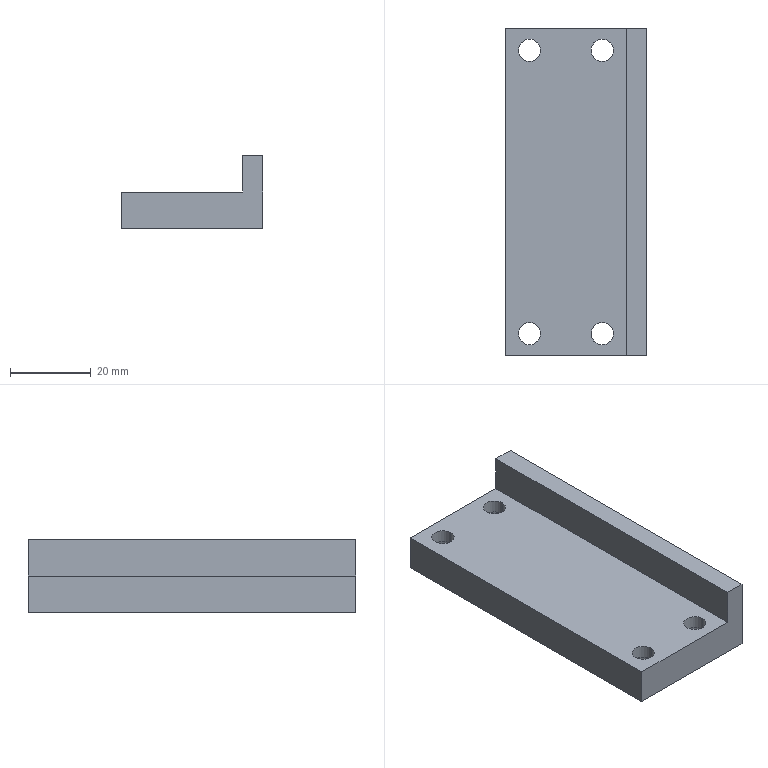Part | STEP file | 1 solid | 28 faces | box 35 x 81 x 18 mm | volume 27056 mm3 | cylinder 16 | plane 12 | commonest cylinder face diameters 5.5 x8 10 x8